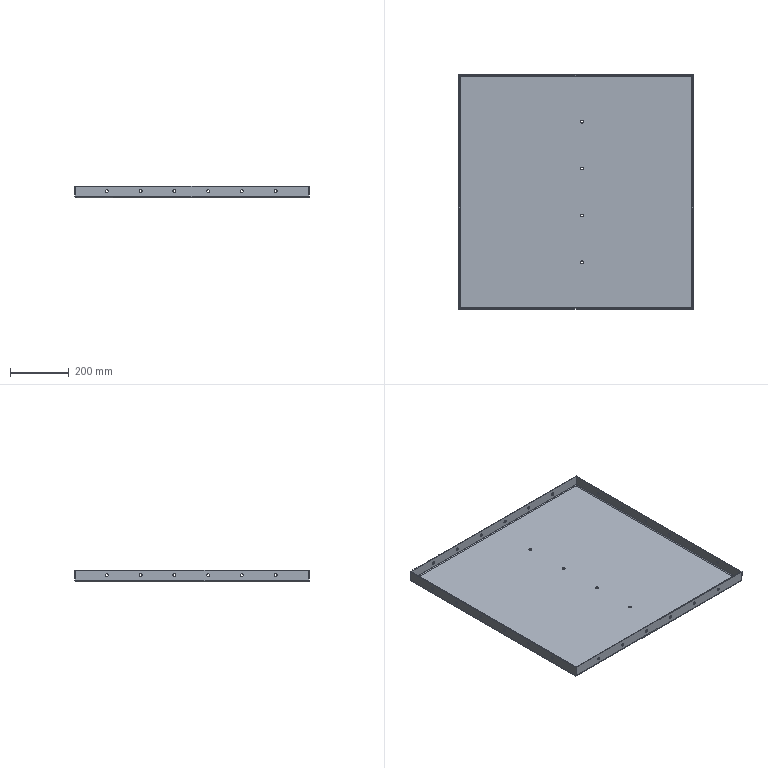Part | SolidWorks | features ICE 3, CornerFeat 1, EdgeFlange 1, FlatPattern 1, SMBaseFlange 1, SheetMetal 1 | 1 solid | 94 faces | box 800 x 800 x 40 mm | volume 2248588 mm3 | cylinder 64 | plane 22 | spline 8 | commonest cylinder face diameters 10 x56 6 x4 12 x4